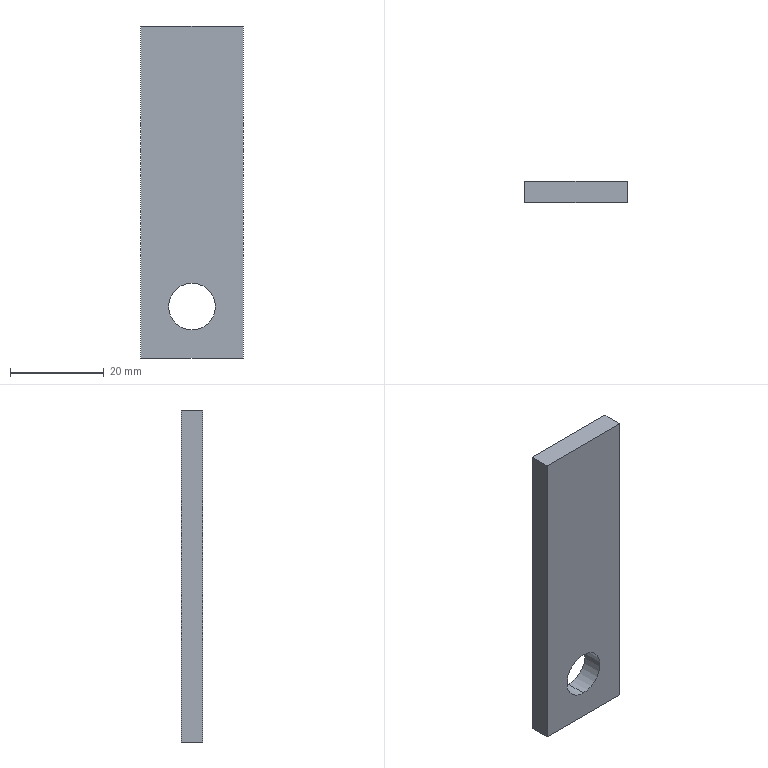Part | SolidWorks | features Extrusion 1 | 1 solid | 8 faces | box 22 x 4.5 x 71 mm | volume 6676 mm3 | plane 6 | cylinder 2 | commonest cylinder face diameters 10 x2
STEP:
#1=CARTESIAN_POINT('',(11.,4.5,-65.));
#2=VERTEX_POINT('',#1);
#3=CARTESIAN_POINT('',(11.,4.5,-55.));
#4=VERTEX_POINT('',#3);
#5=CARTESIAN_POINT('',(11.,4.5,-60.));
#6=DIRECTION('',(0.,1.,0.));
#7=DIRECTION('',(0.,0.,1.));
#8=AXIS2_PLACEMENT_3D('',#5,#6,#7);
#9=CIRCLE('',#8,5.);
#10=EDGE_CURVE('',#2,#4,#9,.T.);
#11=ORIENTED_EDGE('',*,*,#10,.T.);
#12=CARTESIAN_POINT('',(11.,0.,-55.));
#13=VERTEX_POINT('',#12);
#14=CARTESIAN_POINT('',(11.,4.5,-55.));
#15=DIRECTION('',(0.,-1.,0.));
#16=VECTOR('',#15,1000.);
#17=LINE('',#14,#16);
#18=EDGE_CURVE('',#4,#13,#17,.T.);
#19=ORIENTED_EDGE('',*,*,#18,.T.);
#20=CARTESIAN_POINT('',(11.,0.,-65.));
#21=VERTEX_POINT('',#20);
#22=CARTESIAN_POINT('',(11.,0.,-60.));
#23=DIRECTION('',(0.,1.,0.));
#24=DIRECTION('',(0.,0.,1.));
#25=AXIS2_PLACEMENT_3D('',#22,#23,#24);
#26=CIRCLE('',#25,5.);
#27=EDGE_CURVE('',#21,#13,#26,.T.);
#28=ORIENTED_EDGE('',*,*,#27,.F.);
#29=CARTESIAN_POINT('',(11.,4.5,-65.));
#30=DIRECTION('',(0.,-1.,0.));
#31=VECTOR('',#30,1000.);
#32=LINE('',#29,#31);
#33=EDGE_CURVE('',#2,#21,#32,.T.);
#34=ORIENTED_EDGE('',*,*,#33,.F.);
#35=EDGE_LOOP('',(#11,#19,#28,#34));
#36=FACE_OUTER_BOUND('',#35,.T.);
#37=CARTESIAN_POINT('',(11.,4.5,-60.));
#38=DIRECTION('',(0.,-1.,0.));
#39=DIRECTION('',(0.,0.,-1.));
#40=AXIS2_PLACEMENT_3D('',#37,#38,#39);
#41=CYLINDRICAL_SURFACE('',#40,5.);
#42=ADVANCED_FACE('',(#36),#41,.F.);
#43=CARTESIAN_POINT('',(0.,4.5,-71.));
#44=VERTEX_POINT('',#43);
#45=CARTESIAN_POINT('',(0.,4.5,0.));
#46=VERTEX_POINT('',#45);
#47=CARTESIAN_POINT('',(0.,4.5,0.));
#48=DIRECTION('',(0.,0.,1.));
#49=VECTOR('',#48,1000.);
#50=LINE('',#47,#49);
#51=EDGE_CURVE('',#44,#46,#50,.T.);
#52=ORIENTED_EDGE('',*,*,#51,.T.);
#53=CARTESIAN_POINT('',(22.,4.5,0.));
#54=VERTEX_POINT('',#53);
#55=CARTESIAN_POINT('',(0.,4.5,0.));
#56=DIRECTION('',(1.,0.,0.));
#57=VECTOR('',#56,1000.);
#58=LINE('',#55,#57);
#59=EDGE_CURVE('',#46,#54,#58,.T.);
#60=ORIENTED_EDGE('',*,*,#59,.T.);
#61=CARTESIAN_POINT('',(22.,4.5,-71.));
#62=VERTEX_POINT('',#61);
#63=CARTESIAN_POINT('',(22.,4.5,0.));
#64=DIRECTION('',(0.,0.,-1.));
#65=VECTOR('',#64,1000.);
#66=LINE('',#63,#65);
#67=EDGE_CURVE('',#54,#62,#66,.T.);
#68=ORIENTED_EDGE('',*,*,#67,.T.);
#69=CARTESIAN_POINT('',(0.,4.5,-71.));
#70=DIRECTION('',(-1.,0.,0.));
#71=VECTOR('',#70,1000.);
#72=LINE('',#69,#71);
#73=EDGE_CURVE('',#62,#44,#72,.T.);
#74=ORIENTED_EDGE('',*,*,#73,.T.);
#75=EDGE_LOOP('',(#52,#60,#68,#74));
#76=FACE_OUTER_BOUND('',#75,.T.);
#77=ORIENTED_EDGE('',*,*,#10,.F.);
#78=CARTESIAN_POINT('',(11.,4.5,-60.));
#79=DIRECTION('',(0.,1.,0.));
#80=DIRECTION('',(0.,0.,1.));
#81=AXIS2_PLACEMENT_3D('',#78,#79,#80);
#82=CIRCLE('',#81,5.);
#83=EDGE_CURVE('',#4,#2,#82,.T.);
#84=ORIENTED_EDGE('',*,*,#83,.F.);
#85=EDGE_LOOP('',(#77,#84));
#86=FACE_BOUND('',#85,.T.);
#87=CARTESIAN_POINT('',(0.,4.5,0.));
#88=DIRECTION('',(0.,-1.,0.));
#89=DIRECTION('',(0.,0.,-1.));
#90=AXIS2_PLACEMENT_3D('',#87,#88,#89);
#91=PLANE('',#90);
#92=ADVANCED_FACE('',(#76,#86),#91,.F.);
#93=CARTESIAN_POINT('',(0.,0.,-71.));
#94=VERTEX_POINT('',#93);
#95=CARTESIAN_POINT('',(0.,0.,0.));
#96=VERTEX_POINT('',#95);
#97=CARTESIAN_POINT('',(0.,0.,0.));
#98=DIRECTION('',(0.,0.,1.));
#99=VECTOR('',#98,1000.);
#100=LINE('',#97,#99);
#101=EDGE_CURVE('',#94,#96,#100,.T.);
#102=ORIENTED_EDGE('',*,*,#101,.F.);
#103=CARTESIAN_POINT('',(22.,0.,-71.));
#104=VERTEX_POINT('',#103);
#105=CARTESIAN_POINT('',(0.,0.,-71.));
#106=DIRECTION('',(-1.,0.,0.));
#107=VECTOR('',#106,1000.);
#108=LINE('',#105,#107);
#109=EDGE_CURVE('',#104,#94,#108,.T.);
#110=ORIENTED_EDGE('',*,*,#109,.F.);
#111=CARTESIAN_POINT('',(22.,0.,0.));
#112=VERTEX_POINT('',#111);
#113=CARTESIAN_POINT('',(22.,0.,0.));
#114=DIRECTION('',(0.,0.,-1.));
#115=VECTOR('',#114,1000.);
#116=LINE('',#113,#115);
#117=EDGE_CURVE('',#112,#104,#116,.T.);
#118=ORIENTED_EDGE('',*,*,#117,.F.);
#119=CARTESIAN_POINT('',(0.,0.,0.));
#120=DIRECTION('',(1.,0.,0.));
#121=VECTOR('',#120,1000.);
#122=LINE('',#119,#121);
#123=EDGE_CURVE('',#96,#112,#122,.T.);
#124=ORIENTED_EDGE('',*,*,#123,.F.);
#125=EDGE_LOOP('',(#102,#110,#118,#124));
#126=FACE_OUTER_BOUND('',#125,.T.);
#127=ORIENTED_EDGE('',*,*,#27,.T.);
#128=CARTESIAN_POINT('',(11.,0.,-60.));
#129=DIRECTION('',(0.,1.,0.));
#130=DIRECTION('',(0.,0.,1.));
#131=AXIS2_PLACEMENT_3D('',#128,#129,#130);
#132=CIRCLE('',#131,5.);
#133=EDGE_CURVE('',#13,#21,#132,.T.);
#134=ORIENTED_EDGE('',*,*,#133,.T.);
#135=EDGE_LOOP('',(#127,#134));
#136=FACE_BOUND('',#135,.T.);
#137=CARTESIAN_POINT('',(0.,0.,0.));
#138=DIRECTION('',(0.,-1.,0.));
#139=DIRECTION('',(0.,0.,-1.));
#140=AXIS2_PLACEMENT_3D('',#137,#138,#139);
#141=PLANE('',#140);
#142=ADVANCED_FACE('',(#126,#136),#141,.T.);
#143=ORIENTED_EDGE('',*,*,#101,.T.);
#144=CARTESIAN_POINT('',(0.,4.5,0.));
#145=DIRECTION('',(0.,-1.,0.));
#146=VECTOR('',#145,1000.);
#147=LINE('',#144,#146);
#148=EDGE_CURVE('',#46,#96,#147,.T.);
#149=ORIENTED_EDGE('',*,*,#148,.F.);
#150=ORIENTED_EDGE('',*,*,#51,.F.);
#151=CARTESIAN_POINT('',(0.,4.5,-71.));
#152=DIRECTION('',(0.,-1.,0.));
#153=VECTOR('',#152,1000.);
#154=LINE('',#151,#153);
#155=EDGE_CURVE('',#44,#94,#154,.T.);
#156=ORIENTED_EDGE('',*,*,#155,.T.);
#157=EDGE_LOOP('',(#143,#149,#150,#156));
#158=FACE_OUTER_BOUND('',#157,.T.);
#159=CARTESIAN_POINT('',(0.,4.5,0.));
#160=DIRECTION('',(1.,0.,0.));
#161=DIRECTION('',(0.,0.,-1.));
#162=AXIS2_PLACEMENT_3D('',#159,#160,#161);
#163=PLANE('',#162);
#164=ADVANCED_FACE('',(#158),#163,.F.);
#165=ORIENTED_EDGE('',*,*,#123,.T.);
#166=CARTESIAN_POINT('',(22.,4.5,0.));
#167=DIRECTION('',(0.,-1.,0.));
#168=VECTOR('',#167,1000.);
#169=LINE('',#166,#168);
#170=EDGE_CURVE('',#54,#112,#169,.T.);
#171=ORIENTED_EDGE('',*,*,#170,.F.);
#172=ORIENTED_EDGE('',*,*,#59,.F.);
#173=ORIENTED_EDGE('',*,*,#148,.T.);
#174=EDGE_LOOP('',(#165,#171,#172,#173));
#175=FACE_OUTER_BOUND('',#174,.T.);
#176=CARTESIAN_POINT('',(0.,4.5,0.));
#177=DIRECTION('',(0.,0.,-1.));
#178=DIRECTION('',(-1.,0.,0.));
#179=AXIS2_PLACEMENT_3D('',#176,#177,#178);
#180=PLANE('',#179);
#181=ADVANCED_FACE('',(#175),#180,.F.);
#182=ORIENTED_EDGE('',*,*,#117,.T.);
#183=CARTESIAN_POINT('',(22.,4.5,-71.));
#184=DIRECTION('',(0.,-1.,0.));
#185=VECTOR('',#184,1000.);
#186=LINE('',#183,#185);
#187=EDGE_CURVE('',#62,#104,#186,.T.);
#188=ORIENTED_EDGE('',*,*,#187,.F.);
#189=ORIENTED_EDGE('',*,*,#67,.F.);
#190=ORIENTED_EDGE('',*,*,#170,.T.);
#191=EDGE_LOOP('',(#182,#188,#189,#190));
#192=FACE_OUTER_BOUND('',#191,.T.);
#193=CARTESIAN_POINT('',(22.,4.5,0.));
#194=DIRECTION('',(-1.,0.,0.));
#195=DIRECTION('',(0.,0.,1.));
#196=AXIS2_PLACEMENT_3D('',#193,#194,#195);
#197=PLANE('',#196);
#198=ADVANCED_FACE('',(#192),#197,.F.);
#199=ORIENTED_EDGE('',*,*,#109,.T.);
#200=ORIENTED_EDGE('',*,*,#155,.F.);
#201=ORIENTED_EDGE('',*,*,#73,.F.);
#202=ORIENTED_EDGE('',*,*,#187,.T.);
#203=EDGE_LOOP('',(#199,#200,#201,#202));
#204=FACE_OUTER_BOUND('',#203,.T.);
#205=CARTESIAN_POINT('',(0.,4.5,-71.));
#206=DIRECTION('',(0.,0.,1.));
#207=DIRECTION('',(1.,0.,0.));
#208=AXIS2_PLACEMENT_3D('',#205,#206,#207);
#209=PLANE('',#208);
#210=ADVANCED_FACE('',(#204),#209,.F.);
#211=ORIENTED_EDGE('',*,*,#18,.F.);
#212=ORIENTED_EDGE('',*,*,#83,.T.);
#213=ORIENTED_EDGE('',*,*,#33,.T.);
#214=ORIENTED_EDGE('',*,*,#133,.F.);
#215=EDGE_LOOP('',(#211,#212,#213,#214));
#216=FACE_OUTER_BOUND('',#215,.T.);
#217=CARTESIAN_POINT('',(11.,4.5,-60.));
#218=DIRECTION('',(0.,-1.,0.));
#219=DIRECTION('',(0.,0.,-1.));
#220=AXIS2_PLACEMENT_3D('',#217,#218,#219);
#221=CYLINDRICAL_SURFACE('',#220,5.);
#222=ADVANCED_FACE('',(#216),#221,.F.);
#223=CLOSED_SHELL('',(#42,#92,#142,#164,#181,#198,#210,#222));
#224=MANIFOLD_SOLID_BREP('',#223);
#225=CARTESIAN_POINT('',(0.,0.,0.));
#226=DIRECTION('',(0.,0.,1.));
#227=DIRECTION('',(1.,0.,0.));
#228=AXIS2_PLACEMENT_3D('',#225,#226,#227);
#229=(LENGTH_UNIT()NAMED_UNIT(*)SI_UNIT(.MILLI.,.METRE.));
#230=UNCERTAINTY_MEASURE_WITH_UNIT(LENGTH_MEASURE(0.00001),#229,'','');
#231=(NAMED_UNIT(*)PLANE_ANGLE_UNIT()SI_UNIT($,.RADIAN.));
#232=(NAMED_UNIT(*)SI_UNIT($,.STERADIAN.)SOLID_ANGLE_UNIT());
#233=(GEOMETRIC_REPRESENTATION_CONTEXT(3)GLOBAL_UNCERTAINTY_ASSIGNED_CONTEXT((#230))GLOBAL_UNIT_ASSIGNED_CONTEXT((#229,#231,#232))REPRESENTATION_CONTEXT('',''));
#234=ADVANCED_BREP_SHAPE_REPRESENTATION('',(#224,#228),#233);